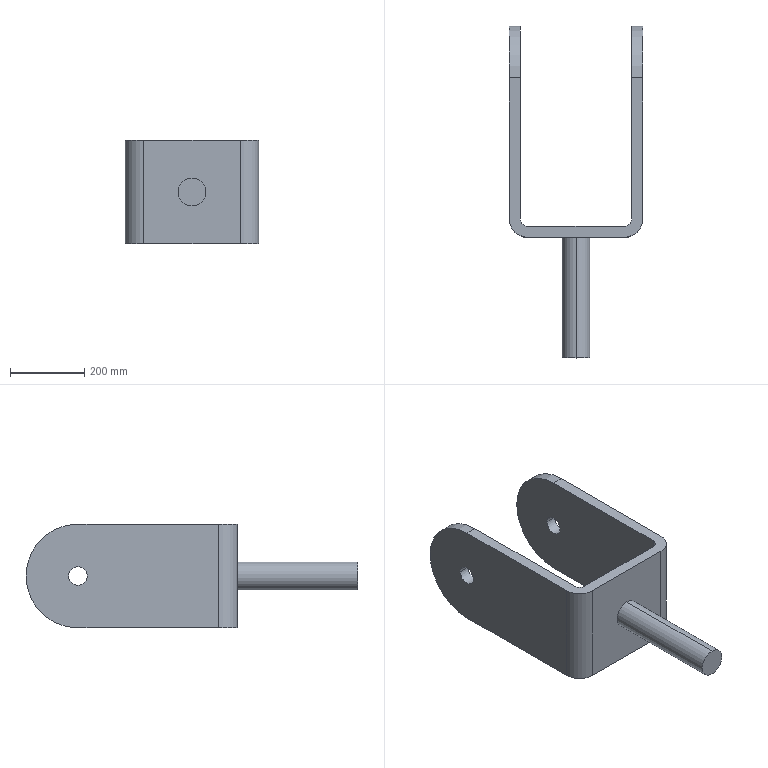Part | SolidWorks | features ICE 6, Extrusion 1, Fillet 1 | 1 solid | 22 faces | box 360 x 895 x 280 mm | volume 12656881 mm3 | cylinder 13 | plane 9 | commonest cylinder face diameters 50 x4 280 x3 40 x2 75 x2 100 x2
STEP:
#1=CARTESIAN_POINT('',(180.,375.,140.));
#2=VERTEX_POINT('',#1);
#3=CARTESIAN_POINT('',(180.,425.,140.));
#4=VERTEX_POINT('',#3);
#5=CARTESIAN_POINT('',(180.,400.,140.));
#6=DIRECTION('',(1.,0.,0.));
#7=DIRECTION('',(0.,-1.,0.));
#8=AXIS2_PLACEMENT_3D('',#5,#6,#7);
#9=CIRCLE('',#8,25.);
#10=EDGE_CURVE('',#2,#4,#9,.T.);
#11=ORIENTED_EDGE('',*,*,#10,.T.);
#12=CARTESIAN_POINT('',(150.,425.,140.));
#13=VERTEX_POINT('',#12);
#14=CARTESIAN_POINT('',(250.711,425.,140.));
#15=DIRECTION('',(-1.,0.,0.));
#16=VECTOR('',#15,1000.);
#17=LINE('',#14,#16);
#18=EDGE_CURVE('',#4,#13,#17,.T.);
#19=ORIENTED_EDGE('',*,*,#18,.T.);
#20=CARTESIAN_POINT('',(150.,375.,140.));
#21=VERTEX_POINT('',#20);
#22=CARTESIAN_POINT('',(150.,400.,140.));
#23=DIRECTION('',(1.,0.,0.));
#24=DIRECTION('',(0.,1.,0.));
#25=AXIS2_PLACEMENT_3D('',#22,#23,#24);
#26=CIRCLE('',#25,25.);
#27=EDGE_CURVE('',#21,#13,#26,.T.);
#28=ORIENTED_EDGE('',*,*,#27,.F.);
#29=CARTESIAN_POINT('',(250.711,375.,140.));
#30=DIRECTION('',(-1.,0.,0.));
#31=VECTOR('',#30,1000.);
#32=LINE('',#29,#31);
#33=EDGE_CURVE('',#2,#21,#32,.T.);
#34=ORIENTED_EDGE('',*,*,#33,.F.);
#35=EDGE_LOOP('',(#11,#19,#28,#34));
#36=FACE_OUTER_BOUND('',#35,.T.);
#37=CARTESIAN_POINT('',(250.711,400.,140.));
#38=DIRECTION('',(-1.,0.,0.));
#39=DIRECTION('',(0.,-1.,0.));
#40=AXIS2_PLACEMENT_3D('',#37,#38,#39);
#41=CYLINDRICAL_SURFACE('',#40,25.);
#42=ADVANCED_FACE('',(#36),#41,.F.);
#43=CARTESIAN_POINT('',(-150.,425.,140.));
#44=VERTEX_POINT('',#43);
#45=CARTESIAN_POINT('',(-150.,375.,140.));
#46=VERTEX_POINT('',#45);
#47=CARTESIAN_POINT('',(-150.,400.,140.));
#48=DIRECTION('',(-1.,0.,0.));
#49=DIRECTION('',(0.,-1.,0.));
#50=AXIS2_PLACEMENT_3D('',#47,#48,#49);
#51=CIRCLE('',#50,25.);
#52=EDGE_CURVE('',#44,#46,#51,.T.);
#53=ORIENTED_EDGE('',*,*,#52,.F.);
#54=CARTESIAN_POINT('',(-180.,425.,140.));
#55=VERTEX_POINT('',#54);
#56=CARTESIAN_POINT('',(250.711,425.,140.));
#57=DIRECTION('',(-1.,0.,0.));
#58=VECTOR('',#57,1000.);
#59=LINE('',#56,#58);
#60=EDGE_CURVE('',#44,#55,#59,.T.);
#61=ORIENTED_EDGE('',*,*,#60,.T.);
#62=CARTESIAN_POINT('',(-180.,375.,140.));
#63=VERTEX_POINT('',#62);
#64=CARTESIAN_POINT('',(-180.,400.,140.));
#65=DIRECTION('',(-1.,0.,0.));
#66=DIRECTION('',(0.,-1.,0.));
#67=AXIS2_PLACEMENT_3D('',#64,#65,#66);
#68=CIRCLE('',#67,25.);
#69=EDGE_CURVE('',#55,#63,#68,.T.);
#70=ORIENTED_EDGE('',*,*,#69,.T.);
#71=CARTESIAN_POINT('',(250.711,375.,140.));
#72=DIRECTION('',(-1.,0.,0.));
#73=VECTOR('',#72,1000.);
#74=LINE('',#71,#73);
#75=EDGE_CURVE('',#46,#63,#74,.T.);
#76=ORIENTED_EDGE('',*,*,#75,.F.);
#77=EDGE_LOOP('',(#53,#61,#70,#76));
#78=FACE_OUTER_BOUND('',#77,.T.);
#79=CARTESIAN_POINT('',(250.711,400.,140.));
#80=DIRECTION('',(-1.,0.,0.));
#81=DIRECTION('',(0.,-1.,0.));
#82=AXIS2_PLACEMENT_3D('',#79,#80,#81);
#83=CYLINDRICAL_SURFACE('',#82,25.);
#84=ADVANCED_FACE('',(#78),#83,.F.);
#85=CARTESIAN_POINT('',(0.,-355.,102.5));
#86=VERTEX_POINT('',#85);
#87=CARTESIAN_POINT('',(0.,-355.,177.5));
#88=VERTEX_POINT('',#87);
#89=CARTESIAN_POINT('',(0.,-355.,140.));
#90=DIRECTION('',(0.,-1.,0.));
#91=DIRECTION('',(0.,0.,-1.));
#92=AXIS2_PLACEMENT_3D('',#89,#90,#91);
#93=CIRCLE('',#92,37.5);
#94=EDGE_CURVE('',#86,#88,#93,.T.);
#95=ORIENTED_EDGE('',*,*,#94,.F.);
#96=CARTESIAN_POINT('',(0.,-30.,102.5));
#97=VERTEX_POINT('',#96);
#98=CARTESIAN_POINT('',(0.,-355.,102.5));
#99=DIRECTION('',(0.,1.,0.));
#100=VECTOR('',#99,1000.);
#101=LINE('',#98,#100);
#102=EDGE_CURVE('',#86,#97,#101,.T.);
#103=ORIENTED_EDGE('',*,*,#102,.T.);
#104=CARTESIAN_POINT('',(0.,-30.,177.5));
#105=VERTEX_POINT('',#104);
#106=CARTESIAN_POINT('',(0.,-30.,140.));
#107=DIRECTION('',(0.,-1.,0.));
#108=DIRECTION('',(0.,0.,1.));
#109=AXIS2_PLACEMENT_3D('',#106,#107,#108);
#110=CIRCLE('',#109,37.5);
#111=EDGE_CURVE('',#97,#105,#110,.T.);
#112=ORIENTED_EDGE('',*,*,#111,.T.);
#113=CARTESIAN_POINT('',(0.,-355.,177.5));
#114=DIRECTION('',(0.,1.,0.));
#115=VECTOR('',#114,1000.);
#116=LINE('',#113,#115);
#117=EDGE_CURVE('',#88,#105,#116,.T.);
#118=ORIENTED_EDGE('',*,*,#117,.F.);
#119=EDGE_LOOP('',(#95,#103,#112,#118));
#120=FACE_OUTER_BOUND('',#119,.T.);
#121=CARTESIAN_POINT('',(0.,-355.,140.));
#122=DIRECTION('',(0.,1.,0.));
#123=DIRECTION('',(0.,0.,1.));
#124=AXIS2_PLACEMENT_3D('',#121,#122,#123);
#125=CYLINDRICAL_SURFACE('',#124,37.5);
#126=ADVANCED_FACE('',(#120),#125,.T.);
#127=CARTESIAN_POINT('',(150.,540.,140.));
#128=VERTEX_POINT('',#127);
#129=CARTESIAN_POINT('',(150.,400.,0.));
#130=VERTEX_POINT('',#129);
#131=CARTESIAN_POINT('',(150.,400.,140.));
#132=DIRECTION('',(-1.,0.,0.));
#133=DIRECTION('',(0.,1.,0.));
#134=AXIS2_PLACEMENT_3D('',#131,#132,#133);
#135=CIRCLE('',#134,140.);
#136=EDGE_CURVE('',#128,#130,#135,.T.);
#137=ORIENTED_EDGE('',*,*,#136,.F.);
#138=CARTESIAN_POINT('',(180.,540.,140.));
#139=VERTEX_POINT('',#138);
#140=CARTESIAN_POINT('',(-163.05,540.,140.));
#141=DIRECTION('',(1.,0.,0.));
#142=VECTOR('',#141,1000.);
#143=LINE('',#140,#142);
#144=EDGE_CURVE('',#128,#139,#143,.T.);
#145=ORIENTED_EDGE('',*,*,#144,.T.);
#146=CARTESIAN_POINT('',(180.,400.,0.));
#147=VERTEX_POINT('',#146);
#148=CARTESIAN_POINT('',(180.,400.,140.));
#149=DIRECTION('',(1.,0.,0.));
#150=DIRECTION('',(0.,1.,0.));
#151=AXIS2_PLACEMENT_3D('',#148,#149,#150);
#152=CIRCLE('',#151,140.);
#153=EDGE_CURVE('',#147,#139,#152,.T.);
#154=ORIENTED_EDGE('',*,*,#153,.F.);
#155=CARTESIAN_POINT('',(54.222,400.,0.));
#156=DIRECTION('',(1.,0.,0.));
#157=VECTOR('',#156,1000.);
#158=LINE('',#155,#157);
#159=EDGE_CURVE('',#130,#147,#158,.T.);
#160=ORIENTED_EDGE('',*,*,#159,.F.);
#161=EDGE_LOOP('',(#137,#145,#154,#160));
#162=FACE_OUTER_BOUND('',#161,.T.);
#163=CARTESIAN_POINT('',(-163.05,400.,140.));
#164=DIRECTION('',(1.,0.,0.));
#165=DIRECTION('',(0.,1.,0.));
#166=AXIS2_PLACEMENT_3D('',#163,#164,#165);
#167=CYLINDRICAL_SURFACE('',#166,140.);
#168=ADVANCED_FACE('',(#162),#167,.T.);
#169=CARTESIAN_POINT('',(-130.,-30.,0.));
#170=VERTEX_POINT('',#169);
#171=CARTESIAN_POINT('',(130.,-30.,0.));
#172=VERTEX_POINT('',#171);
#173=CARTESIAN_POINT('',(-180.,-30.,0.));
#174=DIRECTION('',(1.,0.,0.));
#175=VECTOR('',#174,1000.);
#176=LINE('',#173,#175);
#177=EDGE_CURVE('',#170,#172,#176,.T.);
#178=ORIENTED_EDGE('',*,*,#177,.T.);
#179=CARTESIAN_POINT('',(130.,-30.,280.));
#180=VERTEX_POINT('',#179);
#181=CARTESIAN_POINT('',(130.,-30.,280.));
#182=DIRECTION('',(0.,0.,1.));
#183=VECTOR('',#182,1000.);
#184=LINE('',#181,#183);
#185=EDGE_CURVE('',#172,#180,#184,.T.);
#186=ORIENTED_EDGE('',*,*,#185,.T.);
#187=CARTESIAN_POINT('',(-130.,-30.,280.));
#188=VERTEX_POINT('',#187);
#189=CARTESIAN_POINT('',(-180.,-30.,280.));
#190=DIRECTION('',(1.,0.,0.));
#191=VECTOR('',#190,1000.);
#192=LINE('',#189,#191);
#193=EDGE_CURVE('',#188,#180,#192,.T.);
#194=ORIENTED_EDGE('',*,*,#193,.F.);
#195=CARTESIAN_POINT('',(-130.,-30.,280.));
#196=DIRECTION('',(0.,0.,-1.));
#197=VECTOR('',#196,1000.);
#198=LINE('',#195,#197);
#199=EDGE_CURVE('',#188,#170,#198,.T.);
#200=ORIENTED_EDGE('',*,*,#199,.T.);
#201=EDGE_LOOP('',(#178,#186,#194,#200));
#202=FACE_OUTER_BOUND('',#201,.T.);
#203=CARTESIAN_POINT('',(0.,-30.,140.));
#204=DIRECTION('',(0.,-1.,0.));
#205=DIRECTION('',(0.,0.,1.));
#206=AXIS2_PLACEMENT_3D('',#203,#204,#205);
#207=CIRCLE('',#206,37.5);
#208=EDGE_CURVE('',#105,#97,#207,.T.);
#209=ORIENTED_EDGE('',*,*,#208,.F.);
#210=ORIENTED_EDGE('',*,*,#111,.F.);
#211=EDGE_LOOP('',(#209,#210));
#212=FACE_BOUND('',#211,.T.);
#213=CARTESIAN_POINT('',(-180.,-30.,280.));
#214=DIRECTION('',(0.,1.,0.));
#215=DIRECTION('',(0.,0.,1.));
#216=AXIS2_PLACEMENT_3D('',#213,#214,#215);
#217=PLANE('',#216);
#218=ADVANCED_FACE('',(#202,#212),#217,.F.);
#219=ORIENTED_EDGE('',*,*,#10,.F.);
#220=CARTESIAN_POINT('',(180.,400.,140.));
#221=DIRECTION('',(1.,0.,0.));
#222=DIRECTION('',(0.,-1.,0.));
#223=AXIS2_PLACEMENT_3D('',#220,#221,#222);
#224=CIRCLE('',#223,25.);
#225=EDGE_CURVE('',#4,#2,#224,.T.);
#226=ORIENTED_EDGE('',*,*,#225,.F.);
#227=EDGE_LOOP('',(#219,#226));
#228=FACE_BOUND('',#227,.T.);
#229=CARTESIAN_POINT('',(180.,20.,0.));
#230=VERTEX_POINT('',#229);
#231=CARTESIAN_POINT('',(180.,490.,0.));
#232=DIRECTION('',(0.,1.,0.));
#233=VECTOR('',#232,1000.);
#234=LINE('',#231,#233);
#235=EDGE_CURVE('',#230,#147,#234,.T.);
#236=ORIENTED_EDGE('',*,*,#235,.T.);
#237=ORIENTED_EDGE('',*,*,#153,.T.);
#238=CARTESIAN_POINT('',(180.,400.,280.));
#239=VERTEX_POINT('',#238);
#240=CARTESIAN_POINT('',(180.,400.,140.));
#241=DIRECTION('',(1.,0.,0.));
#242=DIRECTION('',(0.,1.,0.));
#243=AXIS2_PLACEMENT_3D('',#240,#241,#242);
#244=CIRCLE('',#243,140.);
#245=EDGE_CURVE('',#139,#239,#244,.T.);
#246=ORIENTED_EDGE('',*,*,#245,.T.);
#247=CARTESIAN_POINT('',(180.,20.,280.));
#248=VERTEX_POINT('',#247);
#249=CARTESIAN_POINT('',(180.,490.,280.));
#250=DIRECTION('',(0.,1.,0.));
#251=VECTOR('',#250,1000.);
#252=LINE('',#249,#251);
#253=EDGE_CURVE('',#248,#239,#252,.T.);
#254=ORIENTED_EDGE('',*,*,#253,.F.);
#255=CARTESIAN_POINT('',(180.,20.,280.));
#256=DIRECTION('',(0.,0.,-1.));
#257=VECTOR('',#256,1000.);
#258=LINE('',#255,#257);
#259=EDGE_CURVE('',#248,#230,#258,.T.);
#260=ORIENTED_EDGE('',*,*,#259,.T.);
#261=EDGE_LOOP('',(#236,#237,#246,#254,#260));
#262=FACE_OUTER_BOUND('',#261,.T.);
#263=CARTESIAN_POINT('',(180.,490.,280.));
#264=DIRECTION('',(-1.,0.,0.));
#265=DIRECTION('',(0.,-1.,0.));
#266=AXIS2_PLACEMENT_3D('',#263,#264,#265);
#267=PLANE('',#266);
#268=ADVANCED_FACE('',(#228,#262),#267,.F.);
#269=ORIENTED_EDGE('',*,*,#27,.T.);
#270=CARTESIAN_POINT('',(150.,400.,140.));
#271=DIRECTION('',(1.,0.,0.));
#272=DIRECTION('',(0.,1.,0.));
#273=AXIS2_PLACEMENT_3D('',#270,#271,#272);
#274=CIRCLE('',#273,25.);
#275=EDGE_CURVE('',#13,#21,#274,.T.);
#276=ORIENTED_EDGE('',*,*,#275,.T.);
#277=EDGE_LOOP('',(#269,#276));
#278=FACE_BOUND('',#277,.T.);
#279=CARTESIAN_POINT('',(150.,400.,280.));
#280=VERTEX_POINT('',#279);
#281=CARTESIAN_POINT('',(150.,400.,140.));
#282=DIRECTION('',(-1.,0.,0.));
#283=DIRECTION('',(0.,1.,0.));
#284=AXIS2_PLACEMENT_3D('',#281,#282,#283);
#285=CIRCLE('',#284,140.);
#286=EDGE_CURVE('',#280,#128,#285,.T.);
#287=ORIENTED_EDGE('',*,*,#286,.T.);
#288=ORIENTED_EDGE('',*,*,#136,.T.);
#289=CARTESIAN_POINT('',(150.,20.,0.));
#290=VERTEX_POINT('',#289);
#291=CARTESIAN_POINT('',(150.,20.,0.));
#292=DIRECTION('',(0.,-1.,0.));
#293=VECTOR('',#292,1000.);
#294=LINE('',#291,#293);
#295=EDGE_CURVE('',#130,#290,#294,.T.);
#296=ORIENTED_EDGE('',*,*,#295,.T.);
#297=CARTESIAN_POINT('',(150.,20.,280.));
#298=VERTEX_POINT('',#297);
#299=CARTESIAN_POINT('',(150.,20.,280.));
#300=DIRECTION('',(0.,0.,-1.));
#301=VECTOR('',#300,1000.);
#302=LINE('',#299,#301);
#303=EDGE_CURVE('',#298,#290,#302,.T.);
#304=ORIENTED_EDGE('',*,*,#303,.F.);
#305=CARTESIAN_POINT('',(150.,20.,280.));
#306=DIRECTION('',(0.,-1.,0.));
#307=VECTOR('',#306,1000.);
#308=LINE('',#305,#307);
#309=EDGE_CURVE('',#280,#298,#308,.T.);
#310=ORIENTED_EDGE('',*,*,#309,.F.);
#311=EDGE_LOOP('',(#287,#288,#296,#304,#310));
#312=FACE_OUTER_BOUND('',#311,.T.);
#313=CARTESIAN_POINT('',(150.,20.,280.));
#314=DIRECTION('',(1.,0.,0.));
#315=DIRECTION('',(0.,1.,0.));
#316=AXIS2_PLACEMENT_3D('',#313,#314,#315);
#317=PLANE('',#316);
#318=ADVANCED_FACE('',(#278,#312),#317,.F.);
#319=CARTESIAN_POINT('',(-180.,400.,140.));
#320=DIRECTION('',(-1.,0.,0.));
#321=DIRECTION('',(0.,-1.,0.));
#322=AXIS2_PLACEMENT_3D('',#319,#320,#321);
#323=CIRCLE('',#322,25.);
#324=EDGE_CURVE('',#63,#55,#323,.T.);
#325=ORIENTED_EDGE('',*,*,#324,.F.);
#326=ORIENTED_EDGE('',*,*,#69,.F.);
#327=EDGE_LOOP('',(#325,#326));
#328=FACE_BOUND('',#327,.T.);
#329=CARTESIAN_POINT('',(-180.,400.,280.));
#330=VERTEX_POINT('',#329);
#331=CARTESIAN_POINT('',(-180.,20.,280.));
#332=VERTEX_POINT('',#331);
#333=CARTESIAN_POINT('',(-180.,490.,280.));
#334=DIRECTION('',(0.,-1.,0.));
#335=VECTOR('',#334,1000.);
#336=LINE('',#333,#335);
#337=EDGE_CURVE('',#330,#332,#336,.T.);
#338=ORIENTED_EDGE('',*,*,#337,.F.);
#339=CARTESIAN_POINT('',(-180.,400.,0.));
#340=VERTEX_POINT('',#339);
#341=CARTESIAN_POINT('',(-180.,400.,140.));
#342=DIRECTION('',(-1.,0.,0.));
#343=DIRECTION('',(0.,-1.,0.));
#344=AXIS2_PLACEMENT_3D('',#341,#342,#343);
#345=CIRCLE('',#344,140.);
#346=EDGE_CURVE('',#330,#340,#345,.T.);
#347=ORIENTED_EDGE('',*,*,#346,.T.);
#348=CARTESIAN_POINT('',(-180.,20.,0.));
#349=VERTEX_POINT('',#348);
#350=CARTESIAN_POINT('',(-180.,490.,0.));
#351=DIRECTION('',(0.,-1.,0.));
#352=VECTOR('',#351,1000.);
#353=LINE('',#350,#352);
#354=EDGE_CURVE('',#340,#349,#353,.T.);
#355=ORIENTED_EDGE('',*,*,#354,.T.);
#356=CARTESIAN_POINT('',(-180.,20.,280.));
#357=DIRECTION('',(0.,0.,1.));
#358=VECTOR('',#357,1000.);
#359=LINE('',#356,#358);
#360=EDGE_CURVE('',#349,#332,#359,.T.);
#361=ORIENTED_EDGE('',*,*,#360,.T.);
#362=EDGE_LOOP('',(#338,#347,#355,#361));
#363=FACE_OUTER_BOUND('',#362,.T.);
#364=CARTESIAN_POINT('',(-180.,490.,280.));
#365=DIRECTION('',(1.,0.,0.));
#366=DIRECTION('',(0.,1.,0.));
#367=AXIS2_PLACEMENT_3D('',#364,#365,#366);
#368=PLANE('',#367);
#369=ADVANCED_FACE('',(#328,#363),#368,.F.);
#370=CARTESIAN_POINT('',(-150.,400.,140.));
#371=DIRECTION('',(-1.,0.,0.));
#372=DIRECTION('',(0.,-1.,0.));
#373=AXIS2_PLACEMENT_3D('',#370,#371,#372);
#374=CIRCLE('',#373,25.);
#375=EDGE_CURVE('',#46,#44,#374,.T.);
#376=ORIENTED_EDGE('',*,*,#375,.T.);
#377=ORIENTED_EDGE('',*,*,#52,.T.);
#378=EDGE_LOOP('',(#376,#377));
#379=FACE_BOUND('',#378,.T.);
#380=CARTESIAN_POINT('',(-150.,400.,0.));
#381=VERTEX_POINT('',#380);
#382=CARTESIAN_POINT('',(-150.,400.,280.));
#383=VERTEX_POINT('',#382);
#384=CARTESIAN_POINT('',(-150.,400.,140.));
#385=DIRECTION('',(1.,0.,0.));
#386=DIRECTION('',(0.,-1.,0.));
#387=AXIS2_PLACEMENT_3D('',#384,#385,#386);
#388=CIRCLE('',#387,140.);
#389=EDGE_CURVE('',#381,#383,#388,.T.);
#390=ORIENTED_EDGE('',*,*,#389,.T.);
#391=CARTESIAN_POINT('',(-150.,20.,280.));
#392=VERTEX_POINT('',#391);
#393=CARTESIAN_POINT('',(-150.,20.,280.));
#394=DIRECTION('',(0.,1.,0.));
#395=VECTOR('',#394,1000.);
#396=LINE('',#393,#395);
#397=EDGE_CURVE('',#392,#383,#396,.T.);
#398=ORIENTED_EDGE('',*,*,#397,.F.);
#399=CARTESIAN_POINT('',(-150.,20.,0.));
#400=VERTEX_POINT('',#399);
#401=CARTESIAN_POINT('',(-150.,20.,280.));
#402=DIRECTION('',(0.,0.,-1.));
#403=VECTOR('',#402,1000.);
#404=LINE('',#401,#403);
#405=EDGE_CURVE('',#392,#400,#404,.T.);
#406=ORIENTED_EDGE('',*,*,#405,.T.);
#407=CARTESIAN_POINT('',(-150.,20.,0.));
#408=DIRECTION('',(0.,1.,0.));
#409=VECTOR('',#408,1000.);
#410=LINE('',#407,#409);
#411=EDGE_CURVE('',#400,#381,#410,.T.);
#412=ORIENTED_EDGE('',*,*,#411,.T.);
#413=EDGE_LOOP('',(#390,#398,#406,#412));
#414=FACE_OUTER_BOUND('',#413,.T.);
#415=CARTESIAN_POINT('',(-150.,20.,280.));
#416=DIRECTION('',(-1.,0.,0.));
#417=DIRECTION('',(0.,-1.,0.));
#418=AXIS2_PLACEMENT_3D('',#415,#416,#417);
#419=PLANE('',#418);
#420=ADVANCED_FACE('',(#379,#414),#419,.F.);
#421=CARTESIAN_POINT('',(54.222,400.,280.));
#422=DIRECTION('',(1.,0.,0.));
#423=VECTOR('',#422,1000.);
#424=LINE('',#421,#423);
#425=EDGE_CURVE('',#280,#239,#424,.T.);
#426=ORIENTED_EDGE('',*,*,#425,.F.);
#427=ORIENTED_EDGE('',*,*,#309,.T.);
#428=CARTESIAN_POINT('',(130.,0.,280.));
#429=VERTEX_POINT('',#428);
#430=CARTESIAN_POINT('',(130.,20.,280.));
#431=DIRECTION('',(0.,0.,-1.));
#432=DIRECTION('',(1.,0.,0.));
#433=AXIS2_PLACEMENT_3D('',#430,#431,#432);
#434=CIRCLE('',#433,20.);
#435=EDGE_CURVE('',#298,#429,#434,.T.);
#436=ORIENTED_EDGE('',*,*,#435,.T.);
#437=CARTESIAN_POINT('',(-130.,0.,280.));
#438=VERTEX_POINT('',#437);
#439=CARTESIAN_POINT('',(130.,0.,280.));
#440=DIRECTION('',(-1.,0.,0.));
#441=VECTOR('',#440,1000.);
#442=LINE('',#439,#441);
#443=EDGE_CURVE('',#429,#438,#442,.T.);
#444=ORIENTED_EDGE('',*,*,#443,.T.);
#445=CARTESIAN_POINT('',(-130.,20.,280.));
#446=DIRECTION('',(0.,0.,-1.));
#447=DIRECTION('',(-1.,0.,0.));
#448=AXIS2_PLACEMENT_3D('',#445,#446,#447);
#449=CIRCLE('',#448,20.);
#450=EDGE_CURVE('',#438,#392,#449,.T.);
#451=ORIENTED_EDGE('',*,*,#450,.T.);
#452=ORIENTED_EDGE('',*,*,#397,.T.);
#453=CARTESIAN_POINT('',(-54.222,400.,280.));
#454=DIRECTION('',(-1.,0.,0.));
#455=VECTOR('',#454,1000.);
#456=LINE('',#453,#455);
#457=EDGE_CURVE('',#383,#330,#456,.T.);
#458=ORIENTED_EDGE('',*,*,#457,.T.);
#459=ORIENTED_EDGE('',*,*,#337,.T.);
#460=CARTESIAN_POINT('',(-130.,20.,280.));
#461=DIRECTION('',(0.,0.,1.));
#462=DIRECTION('',(1.,0.,0.));
#463=AXIS2_PLACEMENT_3D('',#460,#461,#462);
#464=CIRCLE('',#463,50.);
#465=EDGE_CURVE('',#332,#188,#464,.T.);
#466=ORIENTED_EDGE('',*,*,#465,.T.);
#467=ORIENTED_EDGE('',*,*,#193,.T.);
#468=CARTESIAN_POINT('',(130.,20.,280.));
#469=DIRECTION('',(0.,0.,1.));
#470=DIRECTION('',(1.,0.,0.));
#471=AXIS2_PLACEMENT_3D('',#468,#469,#470);
#472=CIRCLE('',#471,50.);
#473=EDGE_CURVE('',#180,#248,#472,.T.);
#474=ORIENTED_EDGE('',*,*,#473,.T.);
#475=ORIENTED_EDGE('',*,*,#253,.T.);
#476=EDGE_LOOP('',(#426,#427,#436,#444,#451,#452,#458,#459,#466,#467,#474,#475));
#477=FACE_OUTER_BOUND('',#476,.T.);
#478=CARTESIAN_POINT('',(130.,20.,280.));
#479=DIRECTION('',(0.,0.,1.));
#480=DIRECTION('',(1.,0.,0.));
#481=AXIS2_PLACEMENT_3D('',#478,#479,#480);
#482=PLANE('',#481);
#483=ADVANCED_FACE('',(#477),#482,.T.);
#484=ORIENTED_EDGE('',*,*,#295,.F.);
#485=ORIENTED_EDGE('',*,*,#159,.T.);
#486=ORIENTED_EDGE('',*,*,#235,.F.);
#487=CARTESIAN_POINT('',(130.,20.,0.));
#488=DIRECTION('',(0.,0.,-1.));
#489=DIRECTION('',(1.,0.,0.));
#490=AXIS2_PLACEMENT_3D('',#487,#488,#489);
#491=CIRCLE('',#490,50.);
#492=EDGE_CURVE('',#230,#172,#491,.T.);
#493=ORIENTED_EDGE('',*,*,#492,.T.);
#494=ORIENTED_EDGE('',*,*,#177,.F.);
#495=CARTESIAN_POINT('',(-130.,20.,0.));
#496=DIRECTION('',(0.,0.,-1.));
#497=DIRECTION('',(1.,0.,0.));
#498=AXIS2_PLACEMENT_3D('',#495,#496,#497);
#499=CIRCLE('',#498,50.);
#500=EDGE_CURVE('',#170,#349,#499,.T.);
#501=ORIENTED_EDGE('',*,*,#500,.T.);
#502=ORIENTED_EDGE('',*,*,#354,.F.);
#503=CARTESIAN_POINT('',(-54.222,400.,0.));
#504=DIRECTION('',(-1.,0.,0.));
#505=VECTOR('',#504,1000.);
#506=LINE('',#503,#505);
#507=EDGE_CURVE('',#381,#340,#506,.T.);
#508=ORIENTED_EDGE('',*,*,#507,.F.);
#509=ORIENTED_EDGE('',*,*,#411,.F.);
#510=CARTESIAN_POINT('',(-130.,0.,0.));
#511=VERTEX_POINT('',#510);
#512=CARTESIAN_POINT('',(-130.,20.,0.));
#513=DIRECTION('',(0.,0.,-1.));
#514=DIRECTION('',(-1.,0.,0.));
#515=AXIS2_PLACEMENT_3D('',#512,#513,#514);
#516=CIRCLE('',#515,20.);
#517=EDGE_CURVE('',#511,#400,#516,.T.);
#518=ORIENTED_EDGE('',*,*,#517,.F.);
#519=CARTESIAN_POINT('',(130.,0.,0.));
#520=VERTEX_POINT('',#519);
#521=CARTESIAN_POINT('',(130.,0.,0.));
#522=DIRECTION('',(-1.,0.,0.));
#523=VECTOR('',#522,1000.);
#524=LINE('',#521,#523);
#525=EDGE_CURVE('',#520,#511,#524,.T.);
#526=ORIENTED_EDGE('',*,*,#525,.F.);
#527=CARTESIAN_POINT('',(130.,20.,0.));
#528=DIRECTION('',(0.,0.,-1.));
#529=DIRECTION('',(1.,0.,0.));
#530=AXIS2_PLACEMENT_3D('',#527,#528,#529);
#531=CIRCLE('',#530,20.);
#532=EDGE_CURVE('',#290,#520,#531,.T.);
#533=ORIENTED_EDGE('',*,*,#532,.F.);
#534=EDGE_LOOP('',(#484,#485,#486,#493,#494,#501,#502,#508,#509,#518,#526,#533));
#535=FACE_OUTER_BOUND('',#534,.T.);
#536=CARTESIAN_POINT('',(130.,20.,0.));
#537=DIRECTION('',(0.,0.,1.));
#538=DIRECTION('',(1.,0.,0.));
#539=AXIS2_PLACEMENT_3D('',#536,#537,#538);
#540=PLANE('',#539);
#541=ADVANCED_FACE('',(#535),#540,.F.);
#542=ORIENTED_EDGE('',*,*,#532,.T.);
#543=CARTESIAN_POINT('',(130.,0.,280.));
#544=DIRECTION('',(0.,0.,-1.));
#545=VECTOR('',#544,1000.);
#546=LINE('',#543,#545);
#547=EDGE_CURVE('',#429,#520,#546,.T.);
#548=ORIENTED_EDGE('',*,*,#547,.F.);
#549=ORIENTED_EDGE('',*,*,#435,.F.);
#550=ORIENTED_EDGE('',*,*,#303,.T.);
#551=EDGE_LOOP('',(#542,#548,#549,#550));
#552=FACE_OUTER_BOUND('',#551,.T.);
#553=CARTESIAN_POINT('',(130.,20.,280.));
#554=DIRECTION('',(0.,0.,-1.));
#555=DIRECTION('',(-1.,0.,0.));
#556=AXIS2_PLACEMENT_3D('',#553,#554,#555);
#557=CYLINDRICAL_SURFACE('',#556,20.);
#558=ADVANCED_FACE('',(#552),#557,.F.);
#559=ORIENTED_EDGE('',*,*,#525,.T.);
#560=CARTESIAN_POINT('',(-130.,0.,280.));
#561=DIRECTION('',(0.,0.,-1.));
#562=VECTOR('',#561,1000.);
#563=LINE('',#560,#562);
#564=EDGE_CURVE('',#438,#511,#563,.T.);
#565=ORIENTED_EDGE('',*,*,#564,.F.);
#566=ORIENTED_EDGE('',*,*,#443,.F.);
#567=ORIENTED_EDGE('',*,*,#547,.T.);
#568=EDGE_LOOP('',(#559,#565,#566,#567));
#569=FACE_OUTER_BOUND('',#568,.T.);
#570=CARTESIAN_POINT('',(130.,0.,280.));
#571=DIRECTION('',(0.,-1.,0.));
#572=DIRECTION('',(0.,0.,-1.));
#573=AXIS2_PLACEMENT_3D('',#570,#571,#572);
#574=PLANE('',#573);
#575=ADVANCED_FACE('',(#569),#574,.F.);
#576=ORIENTED_EDGE('',*,*,#517,.T.);
#577=ORIENTED_EDGE('',*,*,#405,.F.);
#578=ORIENTED_EDGE('',*,*,#450,.F.);
#579=ORIENTED_EDGE('',*,*,#564,.T.);
#580=EDGE_LOOP('',(#576,#577,#578,#579));
#581=FACE_OUTER_BOUND('',#580,.T.);
#582=CARTESIAN_POINT('',(-130.,20.,280.));
#583=DIRECTION('',(0.,0.,-1.));
#584=DIRECTION('',(-1.,0.,0.));
#585=AXIS2_PLACEMENT_3D('',#582,#583,#584);
#586=CYLINDRICAL_SURFACE('',#585,20.);
#587=ADVANCED_FACE('',(#581),#586,.F.);
#588=ORIENTED_EDGE('',*,*,#473,.F.);
#589=ORIENTED_EDGE('',*,*,#185,.F.);
#590=ORIENTED_EDGE('',*,*,#492,.F.);
#591=ORIENTED_EDGE('',*,*,#259,.F.);
#592=EDGE_LOOP('',(#588,#589,#590,#591));
#593=FACE_OUTER_BOUND('',#592,.T.);
#594=CARTESIAN_POINT('',(130.,20.,280.));
#595=DIRECTION('',(0.,0.,-1.));
#596=DIRECTION('',(-1.,0.,0.));
#597=AXIS2_PLACEMENT_3D('',#594,#595,#596);
#598=CYLINDRICAL_SURFACE('',#597,50.);
#599=ADVANCED_FACE('',(#593),#598,.T.);
#600=ORIENTED_EDGE('',*,*,#465,.F.);
#601=ORIENTED_EDGE('',*,*,#360,.F.);
#602=ORIENTED_EDGE('',*,*,#500,.F.);
#603=ORIENTED_EDGE('',*,*,#199,.F.);
#604=EDGE_LOOP('',(#600,#601,#602,#603));
#605=FACE_OUTER_BOUND('',#604,.T.);
#606=CARTESIAN_POINT('',(-130.,20.,280.));
#607=DIRECTION('',(0.,0.,-1.));
#608=DIRECTION('',(-1.,0.,0.));
#609=AXIS2_PLACEMENT_3D('',#606,#607,#608);
#610=CYLINDRICAL_SURFACE('',#609,50.);
#611=ADVANCED_FACE('',(#605),#610,.T.);
#612=ORIENTED_EDGE('',*,*,#346,.F.);
#613=ORIENTED_EDGE('',*,*,#457,.F.);
#614=ORIENTED_EDGE('',*,*,#389,.F.);
#615=ORIENTED_EDGE('',*,*,#507,.T.);
#616=EDGE_LOOP('',(#612,#613,#614,#615));
#617=FACE_OUTER_BOUND('',#616,.T.);
#618=CARTESIAN_POINT('',(163.05,400.,140.));
#619=DIRECTION('',(-1.,0.,0.));
#620=DIRECTION('',(0.,-1.,0.));
#621=AXIS2_PLACEMENT_3D('',#618,#619,#620);
#622=CYLINDRICAL_SURFACE('',#621,140.);
#623=ADVANCED_FACE('',(#617),#622,.T.);
#624=ORIENTED_EDGE('',*,*,#144,.F.);
#625=ORIENTED_EDGE('',*,*,#286,.F.);
#626=ORIENTED_EDGE('',*,*,#425,.T.);
#627=ORIENTED_EDGE('',*,*,#245,.F.);
#628=EDGE_LOOP('',(#624,#625,#626,#627));
#629=FACE_OUTER_BOUND('',#628,.T.);
#630=CARTESIAN_POINT('',(-163.05,400.,140.));
#631=DIRECTION('',(1.,0.,0.));
#632=DIRECTION('',(0.,1.,0.));
#633=AXIS2_PLACEMENT_3D('',#630,#631,#632);
#634=CYLINDRICAL_SURFACE('',#633,140.);
#635=ADVANCED_FACE('',(#629),#634,.T.);
#636=ORIENTED_EDGE('',*,*,#102,.F.);
#637=CARTESIAN_POINT('',(0.,-355.,140.));
#638=DIRECTION('',(0.,-1.,0.));
#639=DIRECTION('',(0.,0.,-1.));
#640=AXIS2_PLACEMENT_3D('',#637,#638,#639);
#641=CIRCLE('',#640,37.5);
#642=EDGE_CURVE('',#88,#86,#641,.T.);
#643=ORIENTED_EDGE('',*,*,#642,.F.);
#644=ORIENTED_EDGE('',*,*,#117,.T.);
#645=ORIENTED_EDGE('',*,*,#208,.T.);
#646=EDGE_LOOP('',(#636,#643,#644,#645));
#647=FACE_OUTER_BOUND('',#646,.T.);
#648=CARTESIAN_POINT('',(0.,-355.,140.));
#649=DIRECTION('',(0.,1.,0.));
#650=DIRECTION('',(0.,0.,1.));
#651=AXIS2_PLACEMENT_3D('',#648,#649,#650);
#652=CYLINDRICAL_SURFACE('',#651,37.5);
#653=ADVANCED_FACE('',(#647),#652,.T.);
#654=ORIENTED_EDGE('',*,*,#642,.T.);
#655=ORIENTED_EDGE('',*,*,#94,.T.);
#656=EDGE_LOOP('',(#654,#655));
#657=FACE_OUTER_BOUND('',#656,.T.);
#658=CARTESIAN_POINT('',(0.,-355.,0.));
#659=DIRECTION('',(0.,-1.,0.));
#660=DIRECTION('',(0.,0.,-1.));
#661=AXIS2_PLACEMENT_3D('',#658,#659,#660);
#662=PLANE('',#661);
#663=ADVANCED_FACE('',(#657),#662,.T.);
#664=ORIENTED_EDGE('',*,*,#60,.F.);
#665=ORIENTED_EDGE('',*,*,#375,.F.);
#666=ORIENTED_EDGE('',*,*,#75,.T.);
#667=ORIENTED_EDGE('',*,*,#324,.T.);
#668=EDGE_LOOP('',(#664,#665,#666,#667));
#669=FACE_OUTER_BOUND('',#668,.T.);
#670=CARTESIAN_POINT('',(250.711,400.,140.));
#671=DIRECTION('',(-1.,0.,0.));
#672=DIRECTION('',(0.,-1.,0.));
#673=AXIS2_PLACEMENT_3D('',#670,#671,#672);
#674=CYLINDRICAL_SURFACE('',#673,25.);
#675=ADVANCED_FACE('',(#669),#674,.F.);
#676=ORIENTED_EDGE('',*,*,#18,.F.);
#677=ORIENTED_EDGE('',*,*,#225,.T.);
#678=ORIENTED_EDGE('',*,*,#33,.T.);
#679=ORIENTED_EDGE('',*,*,#275,.F.);
#680=EDGE_LOOP('',(#676,#677,#678,#679));
#681=FACE_OUTER_BOUND('',#680,.T.);
#682=CARTESIAN_POINT('',(250.711,400.,140.));
#683=DIRECTION('',(-1.,0.,0.));
#684=DIRECTION('',(0.,-1.,0.));
#685=AXIS2_PLACEMENT_3D('',#682,#683,#684);
#686=CYLINDRICAL_SURFACE('',#685,25.);
#687=ADVANCED_FACE('',(#681),#686,.F.);
#688=CLOSED_SHELL('',(#42,#84,#126,#168,#218,#268,#318,#369,#420,#483,#541,#558,#575,#587,#599,#611,#623,#635,#653,#663,#675,#687));
#689=MANIFOLD_SOLID_BREP('',#688);
#690=CARTESIAN_POINT('',(0.,0.,0.));
#691=DIRECTION('',(0.,0.,1.));
#692=DIRECTION('',(1.,0.,0.));
#693=AXIS2_PLACEMENT_3D('',#690,#691,#692);
#694=(LENGTH_UNIT()NAMED_UNIT(*)SI_UNIT(.MILLI.,.METRE.));
#695=UNCERTAINTY_MEASURE_WITH_UNIT(LENGTH_MEASURE(0.00001),#694,'','');
#696=(NAMED_UNIT(*)PLANE_ANGLE_UNIT()SI_UNIT($,.RADIAN.));
#697=(NAMED_UNIT(*)SI_UNIT($,.STERADIAN.)SOLID_ANGLE_UNIT());
#698=(GEOMETRIC_REPRESENTATION_CONTEXT(3)GLOBAL_UNCERTAINTY_ASSIGNED_CONTEXT((#695))GLOBAL_UNIT_ASSIGNED_CONTEXT((#694,#696,#697))REPRESENTATION_CONTEXT('',''));
#699=ADVANCED_BREP_SHAPE_REPRESENTATION('',(#689,#693),#698);